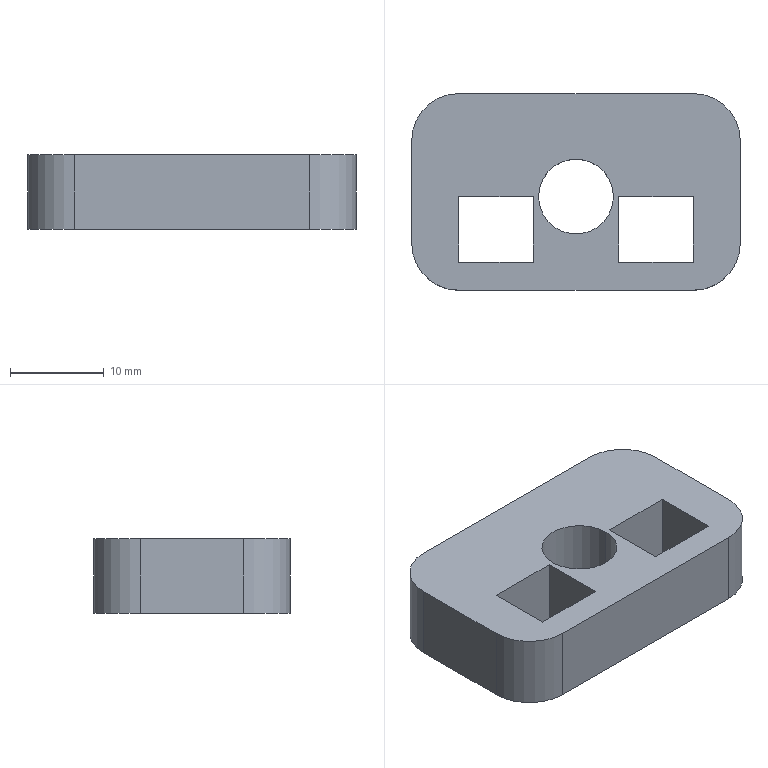Part | SolidWorks | features Fillet 1, FlatPattern 1, SMBaseFlange 1, SheetMetal 1 | 1 solid | 20 faces | box 35.1 x 21 x 8 mm | volume 4427 mm3 | plane 14 | cylinder 6 | commonest cylinder face diameters 10 x4 8 x2
STEP:
#1=CARTESIAN_POINT('',(8.55,26.043,8.));
#2=VERTEX_POINT('',#1);
#3=CARTESIAN_POINT('',(16.55,26.043,8.));
#4=VERTEX_POINT('',#3);
#5=CARTESIAN_POINT('',(12.55,26.043,8.));
#6=DIRECTION('',(0.,0.,1.));
#7=DIRECTION('',(1.,0.,0.));
#8=AXIS2_PLACEMENT_3D('',#5,#6,#7);
#9=CIRCLE('',#8,4.);
#10=EDGE_CURVE('',#2,#4,#9,.T.);
#11=ORIENTED_EDGE('',*,*,#10,.T.);
#12=CARTESIAN_POINT('',(16.55,26.043,0.));
#13=VERTEX_POINT('',#12);
#14=CARTESIAN_POINT('',(16.55,26.043,8.));
#15=DIRECTION('',(0.,0.,-1.));
#16=VECTOR('',#15,1000.);
#17=LINE('',#14,#16);
#18=EDGE_CURVE('',#4,#13,#17,.T.);
#19=ORIENTED_EDGE('',*,*,#18,.T.);
#20=CARTESIAN_POINT('',(8.55,26.043,0.));
#21=VERTEX_POINT('',#20);
#22=CARTESIAN_POINT('',(12.55,26.043,0.));
#23=DIRECTION('',(0.,0.,1.));
#24=DIRECTION('',(1.,0.,0.));
#25=AXIS2_PLACEMENT_3D('',#22,#23,#24);
#26=CIRCLE('',#25,4.);
#27=EDGE_CURVE('',#21,#13,#26,.T.);
#28=ORIENTED_EDGE('',*,*,#27,.F.);
#29=CARTESIAN_POINT('',(8.55,26.043,8.));
#30=DIRECTION('',(0.,0.,-1.));
#31=VECTOR('',#30,1000.);
#32=LINE('',#29,#31);
#33=EDGE_CURVE('',#2,#21,#32,.T.);
#34=ORIENTED_EDGE('',*,*,#33,.F.);
#35=EDGE_LOOP('',(#11,#19,#28,#34));
#36=FACE_OUTER_BOUND('',#35,.T.);
#37=CARTESIAN_POINT('',(12.55,26.043,8.));
#38=DIRECTION('',(0.,0.,-1.));
#39=DIRECTION('',(-1.,0.,0.));
#40=AXIS2_PLACEMENT_3D('',#37,#38,#39);
#41=CYLINDRICAL_SURFACE('',#40,4.);
#42=ADVANCED_FACE('',(#36),#41,.F.);
#43=CARTESIAN_POINT('',(0.,26.043,8.));
#44=VERTEX_POINT('',#43);
#45=CARTESIAN_POINT('',(0.,19.043,8.));
#46=VERTEX_POINT('',#45);
#47=CARTESIAN_POINT('',(0.,19.043,8.));
#48=DIRECTION('',(0.,-1.,0.));
#49=VECTOR('',#48,1000.);
#50=LINE('',#47,#49);
#51=EDGE_CURVE('',#44,#46,#50,.T.);
#52=ORIENTED_EDGE('',*,*,#51,.F.);
#53=CARTESIAN_POINT('',(8.,26.043,8.));
#54=VERTEX_POINT('',#53);
#55=CARTESIAN_POINT('',(0.,26.043,8.));
#56=DIRECTION('',(-1.,0.,0.));
#57=VECTOR('',#56,1000.);
#58=LINE('',#55,#57);
#59=EDGE_CURVE('',#54,#44,#58,.T.);
#60=ORIENTED_EDGE('',*,*,#59,.F.);
#61=CARTESIAN_POINT('',(8.,19.043,8.));
#62=VERTEX_POINT('',#61);
#63=CARTESIAN_POINT('',(8.,19.043,8.));
#64=DIRECTION('',(0.,1.,0.));
#65=VECTOR('',#64,1000.);
#66=LINE('',#63,#65);
#67=EDGE_CURVE('',#62,#54,#66,.T.);
#68=ORIENTED_EDGE('',*,*,#67,.F.);
#69=CARTESIAN_POINT('',(0.,19.043,8.));
#70=DIRECTION('',(1.,0.,0.));
#71=VECTOR('',#70,1000.);
#72=LINE('',#69,#71);
#73=EDGE_CURVE('',#46,#62,#72,.T.);
#74=ORIENTED_EDGE('',*,*,#73,.F.);
#75=EDGE_LOOP('',(#52,#60,#68,#74));
#76=FACE_BOUND('',#75,.T.);
#77=CARTESIAN_POINT('',(25.1,37.043,8.));
#78=VERTEX_POINT('',#77);
#79=CARTESIAN_POINT('',(0.,37.043,8.));
#80=VERTEX_POINT('',#79);
#81=CARTESIAN_POINT('',(-5.,37.043,8.));
#82=DIRECTION('',(-1.,0.,0.));
#83=VECTOR('',#82,1000.);
#84=LINE('',#81,#83);
#85=EDGE_CURVE('',#78,#80,#84,.T.);
#86=ORIENTED_EDGE('',*,*,#85,.T.);
#87=CARTESIAN_POINT('',(-5.,32.043,8.));
#88=VERTEX_POINT('',#87);
#89=CARTESIAN_POINT('',(0.,32.043,8.));
#90=DIRECTION('',(0.,0.,1.));
#91=DIRECTION('',(-1.,0.,0.));
#92=AXIS2_PLACEMENT_3D('',#89,#90,#91);
#93=CIRCLE('',#92,5.);
#94=EDGE_CURVE('',#80,#88,#93,.T.);
#95=ORIENTED_EDGE('',*,*,#94,.T.);
#96=CARTESIAN_POINT('',(-5.,21.043,8.));
#97=VERTEX_POINT('',#96);
#98=CARTESIAN_POINT('',(-5.,16.043,8.));
#99=DIRECTION('',(0.,-1.,0.));
#100=VECTOR('',#99,1000.);
#101=LINE('',#98,#100);
#102=EDGE_CURVE('',#88,#97,#101,.T.);
#103=ORIENTED_EDGE('',*,*,#102,.T.);
#104=CARTESIAN_POINT('',(0.,16.043,8.));
#105=VERTEX_POINT('',#104);
#106=CARTESIAN_POINT('',(0.,21.043,8.));
#107=DIRECTION('',(0.,0.,1.));
#108=DIRECTION('',(-1.,0.,0.));
#109=AXIS2_PLACEMENT_3D('',#106,#107,#108);
#110=CIRCLE('',#109,5.);
#111=EDGE_CURVE('',#97,#105,#110,.T.);
#112=ORIENTED_EDGE('',*,*,#111,.T.);
#113=CARTESIAN_POINT('',(25.1,16.043,8.));
#114=VERTEX_POINT('',#113);
#115=CARTESIAN_POINT('',(-5.,16.043,8.));
#116=DIRECTION('',(1.,0.,0.));
#117=VECTOR('',#116,1000.);
#118=LINE('',#115,#117);
#119=EDGE_CURVE('',#105,#114,#118,.T.);
#120=ORIENTED_EDGE('',*,*,#119,.T.);
#121=CARTESIAN_POINT('',(30.1,21.043,8.));
#122=VERTEX_POINT('',#121);
#123=CARTESIAN_POINT('',(25.1,21.043,8.));
#124=DIRECTION('',(0.,0.,1.));
#125=DIRECTION('',(-1.,0.,0.));
#126=AXIS2_PLACEMENT_3D('',#123,#124,#125);
#127=CIRCLE('',#126,5.);
#128=EDGE_CURVE('',#114,#122,#127,.T.);
#129=ORIENTED_EDGE('',*,*,#128,.T.);
#130=CARTESIAN_POINT('',(30.1,32.043,8.));
#131=VERTEX_POINT('',#130);
#132=CARTESIAN_POINT('',(30.1,16.043,8.));
#133=DIRECTION('',(0.,1.,0.));
#134=VECTOR('',#133,1000.);
#135=LINE('',#132,#134);
#136=EDGE_CURVE('',#122,#131,#135,.T.);
#137=ORIENTED_EDGE('',*,*,#136,.T.);
#138=CARTESIAN_POINT('',(25.1,32.043,8.));
#139=DIRECTION('',(0.,0.,1.));
#140=DIRECTION('',(-1.,0.,0.));
#141=AXIS2_PLACEMENT_3D('',#138,#139,#140);
#142=CIRCLE('',#141,5.);
#143=EDGE_CURVE('',#131,#78,#142,.T.);
#144=ORIENTED_EDGE('',*,*,#143,.T.);
#145=EDGE_LOOP('',(#86,#95,#103,#112,#120,#129,#137,#144));
#146=FACE_OUTER_BOUND('',#145,.T.);
#147=CARTESIAN_POINT('',(17.1,26.043,8.));
#148=VERTEX_POINT('',#147);
#149=CARTESIAN_POINT('',(17.1,19.043,8.));
#150=VERTEX_POINT('',#149);
#151=CARTESIAN_POINT('',(17.1,19.043,8.));
#152=DIRECTION('',(0.,-1.,0.));
#153=VECTOR('',#152,1000.);
#154=LINE('',#151,#153);
#155=EDGE_CURVE('',#148,#150,#154,.T.);
#156=ORIENTED_EDGE('',*,*,#155,.F.);
#157=CARTESIAN_POINT('',(25.1,26.043,8.));
#158=VERTEX_POINT('',#157);
#159=CARTESIAN_POINT('',(17.1,26.043,8.));
#160=DIRECTION('',(-1.,0.,0.));
#161=VECTOR('',#160,1000.);
#162=LINE('',#159,#161);
#163=EDGE_CURVE('',#158,#148,#162,.T.);
#164=ORIENTED_EDGE('',*,*,#163,.F.);
#165=CARTESIAN_POINT('',(25.1,19.043,8.));
#166=VERTEX_POINT('',#165);
#167=CARTESIAN_POINT('',(25.1,19.043,8.));
#168=DIRECTION('',(0.,1.,0.));
#169=VECTOR('',#168,1000.);
#170=LINE('',#167,#169);
#171=EDGE_CURVE('',#166,#158,#170,.T.);
#172=ORIENTED_EDGE('',*,*,#171,.F.);
#173=CARTESIAN_POINT('',(17.1,19.043,8.));
#174=DIRECTION('',(1.,0.,0.));
#175=VECTOR('',#174,1000.);
#176=LINE('',#173,#175);
#177=EDGE_CURVE('',#150,#166,#176,.T.);
#178=ORIENTED_EDGE('',*,*,#177,.F.);
#179=EDGE_LOOP('',(#156,#164,#172,#178));
#180=FACE_BOUND('',#179,.T.);
#181=ORIENTED_EDGE('',*,*,#10,.F.);
#182=CARTESIAN_POINT('',(12.55,26.043,8.));
#183=DIRECTION('',(0.,0.,1.));
#184=DIRECTION('',(1.,0.,0.));
#185=AXIS2_PLACEMENT_3D('',#182,#183,#184);
#186=CIRCLE('',#185,4.);
#187=EDGE_CURVE('',#4,#2,#186,.T.);
#188=ORIENTED_EDGE('',*,*,#187,.F.);
#189=EDGE_LOOP('',(#181,#188));
#190=FACE_BOUND('',#189,.T.);
#191=CARTESIAN_POINT('',(0.,0.,8.));
#192=DIRECTION('',(0.,0.,-1.));
#193=DIRECTION('',(-1.,0.,0.));
#194=AXIS2_PLACEMENT_3D('',#191,#192,#193);
#195=PLANE('',#194);
#196=ADVANCED_FACE('',(#76,#146,#180,#190),#195,.F.);
#197=CARTESIAN_POINT('',(25.1,26.043,0.));
#198=VERTEX_POINT('',#197);
#199=CARTESIAN_POINT('',(17.1,26.043,0.));
#200=VERTEX_POINT('',#199);
#201=CARTESIAN_POINT('',(17.1,26.043,0.));
#202=DIRECTION('',(-1.,0.,0.));
#203=VECTOR('',#202,1000.);
#204=LINE('',#201,#203);
#205=EDGE_CURVE('',#198,#200,#204,.T.);
#206=ORIENTED_EDGE('',*,*,#205,.T.);
#207=CARTESIAN_POINT('',(17.1,19.043,0.));
#208=VERTEX_POINT('',#207);
#209=CARTESIAN_POINT('',(17.1,19.043,0.));
#210=DIRECTION('',(0.,-1.,0.));
#211=VECTOR('',#210,1000.);
#212=LINE('',#209,#211);
#213=EDGE_CURVE('',#200,#208,#212,.T.);
#214=ORIENTED_EDGE('',*,*,#213,.T.);
#215=CARTESIAN_POINT('',(25.1,19.043,0.));
#216=VERTEX_POINT('',#215);
#217=CARTESIAN_POINT('',(17.1,19.043,0.));
#218=DIRECTION('',(1.,0.,0.));
#219=VECTOR('',#218,1000.);
#220=LINE('',#217,#219);
#221=EDGE_CURVE('',#208,#216,#220,.T.);
#222=ORIENTED_EDGE('',*,*,#221,.T.);
#223=CARTESIAN_POINT('',(25.1,19.043,0.));
#224=DIRECTION('',(0.,1.,0.));
#225=VECTOR('',#224,1000.);
#226=LINE('',#223,#225);
#227=EDGE_CURVE('',#216,#198,#226,.T.);
#228=ORIENTED_EDGE('',*,*,#227,.T.);
#229=EDGE_LOOP('',(#206,#214,#222,#228));
#230=FACE_BOUND('',#229,.T.);
#231=CARTESIAN_POINT('',(8.,26.043,0.));
#232=VERTEX_POINT('',#231);
#233=CARTESIAN_POINT('',(0.,26.043,0.));
#234=VERTEX_POINT('',#233);
#235=CARTESIAN_POINT('',(0.,26.043,0.));
#236=DIRECTION('',(-1.,0.,0.));
#237=VECTOR('',#236,1000.);
#238=LINE('',#235,#237);
#239=EDGE_CURVE('',#232,#234,#238,.T.);
#240=ORIENTED_EDGE('',*,*,#239,.T.);
#241=CARTESIAN_POINT('',(0.,19.043,0.));
#242=VERTEX_POINT('',#241);
#243=CARTESIAN_POINT('',(0.,19.043,0.));
#244=DIRECTION('',(0.,-1.,0.));
#245=VECTOR('',#244,1000.);
#246=LINE('',#243,#245);
#247=EDGE_CURVE('',#234,#242,#246,.T.);
#248=ORIENTED_EDGE('',*,*,#247,.T.);
#249=CARTESIAN_POINT('',(8.,19.043,0.));
#250=VERTEX_POINT('',#249);
#251=CARTESIAN_POINT('',(0.,19.043,0.));
#252=DIRECTION('',(1.,0.,0.));
#253=VECTOR('',#252,1000.);
#254=LINE('',#251,#253);
#255=EDGE_CURVE('',#242,#250,#254,.T.);
#256=ORIENTED_EDGE('',*,*,#255,.T.);
#257=CARTESIAN_POINT('',(8.,19.043,0.));
#258=DIRECTION('',(0.,1.,0.));
#259=VECTOR('',#258,1000.);
#260=LINE('',#257,#259);
#261=EDGE_CURVE('',#250,#232,#260,.T.);
#262=ORIENTED_EDGE('',*,*,#261,.T.);
#263=EDGE_LOOP('',(#240,#248,#256,#262));
#264=FACE_BOUND('',#263,.T.);
#265=CARTESIAN_POINT('',(-5.,32.043,0.));
#266=VERTEX_POINT('',#265);
#267=CARTESIAN_POINT('',(-5.,21.043,0.));
#268=VERTEX_POINT('',#267);
#269=CARTESIAN_POINT('',(-5.,16.043,0.));
#270=DIRECTION('',(0.,-1.,0.));
#271=VECTOR('',#270,1000.);
#272=LINE('',#269,#271);
#273=EDGE_CURVE('',#266,#268,#272,.T.);
#274=ORIENTED_EDGE('',*,*,#273,.F.);
#275=CARTESIAN_POINT('',(0.,37.043,0.));
#276=VERTEX_POINT('',#275);
#277=CARTESIAN_POINT('',(0.,32.043,0.));
#278=DIRECTION('',(0.,0.,-1.));
#279=DIRECTION('',(-1.,0.,0.));
#280=AXIS2_PLACEMENT_3D('',#277,#278,#279);
#281=CIRCLE('',#280,5.);
#282=EDGE_CURVE('',#266,#276,#281,.T.);
#283=ORIENTED_EDGE('',*,*,#282,.T.);
#284=CARTESIAN_POINT('',(25.1,37.043,0.));
#285=VERTEX_POINT('',#284);
#286=CARTESIAN_POINT('',(-5.,37.043,0.));
#287=DIRECTION('',(-1.,0.,0.));
#288=VECTOR('',#287,1000.);
#289=LINE('',#286,#288);
#290=EDGE_CURVE('',#285,#276,#289,.T.);
#291=ORIENTED_EDGE('',*,*,#290,.F.);
#292=CARTESIAN_POINT('',(30.1,32.043,0.));
#293=VERTEX_POINT('',#292);
#294=CARTESIAN_POINT('',(25.1,32.043,0.));
#295=DIRECTION('',(0.,0.,-1.));
#296=DIRECTION('',(-1.,0.,0.));
#297=AXIS2_PLACEMENT_3D('',#294,#295,#296);
#298=CIRCLE('',#297,5.);
#299=EDGE_CURVE('',#285,#293,#298,.T.);
#300=ORIENTED_EDGE('',*,*,#299,.T.);
#301=CARTESIAN_POINT('',(30.1,21.043,0.));
#302=VERTEX_POINT('',#301);
#303=CARTESIAN_POINT('',(30.1,16.043,0.));
#304=DIRECTION('',(0.,1.,0.));
#305=VECTOR('',#304,1000.);
#306=LINE('',#303,#305);
#307=EDGE_CURVE('',#302,#293,#306,.T.);
#308=ORIENTED_EDGE('',*,*,#307,.F.);
#309=CARTESIAN_POINT('',(25.1,16.043,0.));
#310=VERTEX_POINT('',#309);
#311=CARTESIAN_POINT('',(25.1,21.043,0.));
#312=DIRECTION('',(0.,0.,-1.));
#313=DIRECTION('',(-1.,0.,0.));
#314=AXIS2_PLACEMENT_3D('',#311,#312,#313);
#315=CIRCLE('',#314,5.);
#316=EDGE_CURVE('',#302,#310,#315,.T.);
#317=ORIENTED_EDGE('',*,*,#316,.T.);
#318=CARTESIAN_POINT('',(0.,16.043,0.));
#319=VERTEX_POINT('',#318);
#320=CARTESIAN_POINT('',(-5.,16.043,0.));
#321=DIRECTION('',(1.,0.,0.));
#322=VECTOR('',#321,1000.);
#323=LINE('',#320,#322);
#324=EDGE_CURVE('',#319,#310,#323,.T.);
#325=ORIENTED_EDGE('',*,*,#324,.F.);
#326=CARTESIAN_POINT('',(0.,21.043,0.));
#327=DIRECTION('',(0.,0.,-1.));
#328=DIRECTION('',(-1.,0.,0.));
#329=AXIS2_PLACEMENT_3D('',#326,#327,#328);
#330=CIRCLE('',#329,5.);
#331=EDGE_CURVE('',#319,#268,#330,.T.);
#332=ORIENTED_EDGE('',*,*,#331,.T.);
#333=EDGE_LOOP('',(#274,#283,#291,#300,#308,#317,#325,#332));
#334=FACE_OUTER_BOUND('',#333,.T.);
#335=ORIENTED_EDGE('',*,*,#27,.T.);
#336=CARTESIAN_POINT('',(12.55,26.043,0.));
#337=DIRECTION('',(0.,0.,1.));
#338=DIRECTION('',(1.,0.,0.));
#339=AXIS2_PLACEMENT_3D('',#336,#337,#338);
#340=CIRCLE('',#339,4.);
#341=EDGE_CURVE('',#13,#21,#340,.T.);
#342=ORIENTED_EDGE('',*,*,#341,.T.);
#343=EDGE_LOOP('',(#335,#342));
#344=FACE_BOUND('',#343,.T.);
#345=CARTESIAN_POINT('',(0.,0.,0.));
#346=DIRECTION('',(0.,0.,-1.));
#347=DIRECTION('',(-1.,0.,0.));
#348=AXIS2_PLACEMENT_3D('',#345,#346,#347);
#349=PLANE('',#348);
#350=ADVANCED_FACE('',(#230,#264,#334,#344),#349,.T.);
#351=ORIENTED_EDGE('',*,*,#102,.F.);
#352=CARTESIAN_POINT('',(-5.,32.043,8.));
#353=DIRECTION('',(0.,0.,-1.));
#354=VECTOR('',#353,1000.);
#355=LINE('',#352,#354);
#356=EDGE_CURVE('',#88,#266,#355,.T.);
#357=ORIENTED_EDGE('',*,*,#356,.T.);
#358=ORIENTED_EDGE('',*,*,#273,.T.);
#359=CARTESIAN_POINT('',(-5.,21.043,8.));
#360=DIRECTION('',(0.,0.,1.));
#361=VECTOR('',#360,1000.);
#362=LINE('',#359,#361);
#363=EDGE_CURVE('',#268,#97,#362,.T.);
#364=ORIENTED_EDGE('',*,*,#363,.T.);
#365=EDGE_LOOP('',(#351,#357,#358,#364));
#366=FACE_OUTER_BOUND('',#365,.T.);
#367=CARTESIAN_POINT('',(-5.,16.043,8.));
#368=DIRECTION('',(1.,0.,0.));
#369=DIRECTION('',(0.,1.,0.));
#370=AXIS2_PLACEMENT_3D('',#367,#368,#369);
#371=PLANE('',#370);
#372=ADVANCED_FACE('',(#366),#371,.F.);
#373=ORIENTED_EDGE('',*,*,#324,.T.);
#374=CARTESIAN_POINT('',(25.1,16.043,8.));
#375=DIRECTION('',(0.,0.,1.));
#376=VECTOR('',#375,1000.);
#377=LINE('',#374,#376);
#378=EDGE_CURVE('',#310,#114,#377,.T.);
#379=ORIENTED_EDGE('',*,*,#378,.T.);
#380=ORIENTED_EDGE('',*,*,#119,.F.);
#381=CARTESIAN_POINT('',(0.,16.043,8.));
#382=DIRECTION('',(0.,0.,-1.));
#383=VECTOR('',#382,1000.);
#384=LINE('',#381,#383);
#385=EDGE_CURVE('',#105,#319,#384,.T.);
#386=ORIENTED_EDGE('',*,*,#385,.T.);
#387=EDGE_LOOP('',(#373,#379,#380,#386));
#388=FACE_OUTER_BOUND('',#387,.T.);
#389=CARTESIAN_POINT('',(-5.,16.043,8.));
#390=DIRECTION('',(0.,1.,0.));
#391=DIRECTION('',(0.,0.,1.));
#392=AXIS2_PLACEMENT_3D('',#389,#390,#391);
#393=PLANE('',#392);
#394=ADVANCED_FACE('',(#388),#393,.F.);
#395=ORIENTED_EDGE('',*,*,#307,.T.);
#396=CARTESIAN_POINT('',(30.1,32.043,8.));
#397=DIRECTION('',(0.,0.,1.));
#398=VECTOR('',#397,1000.);
#399=LINE('',#396,#398);
#400=EDGE_CURVE('',#293,#131,#399,.T.);
#401=ORIENTED_EDGE('',*,*,#400,.T.);
#402=ORIENTED_EDGE('',*,*,#136,.F.);
#403=CARTESIAN_POINT('',(30.1,21.043,8.));
#404=DIRECTION('',(0.,0.,-1.));
#405=VECTOR('',#404,1000.);
#406=LINE('',#403,#405);
#407=EDGE_CURVE('',#122,#302,#406,.T.);
#408=ORIENTED_EDGE('',*,*,#407,.T.);
#409=EDGE_LOOP('',(#395,#401,#402,#408));
#410=FACE_OUTER_BOUND('',#409,.T.);
#411=CARTESIAN_POINT('',(30.1,16.043,8.));
#412=DIRECTION('',(-1.,0.,0.));
#413=DIRECTION('',(0.,0.,1.));
#414=AXIS2_PLACEMENT_3D('',#411,#412,#413);
#415=PLANE('',#414);
#416=ADVANCED_FACE('',(#410),#415,.F.);
#417=ORIENTED_EDGE('',*,*,#290,.T.);
#418=CARTESIAN_POINT('',(0.,37.043,8.));
#419=DIRECTION('',(0.,0.,1.));
#420=VECTOR('',#419,1000.);
#421=LINE('',#418,#420);
#422=EDGE_CURVE('',#276,#80,#421,.T.);
#423=ORIENTED_EDGE('',*,*,#422,.T.);
#424=ORIENTED_EDGE('',*,*,#85,.F.);
#425=CARTESIAN_POINT('',(25.1,37.043,8.));
#426=DIRECTION('',(0.,0.,-1.));
#427=VECTOR('',#426,1000.);
#428=LINE('',#425,#427);
#429=EDGE_CURVE('',#78,#285,#428,.T.);
#430=ORIENTED_EDGE('',*,*,#429,.T.);
#431=EDGE_LOOP('',(#417,#423,#424,#430));
#432=FACE_OUTER_BOUND('',#431,.T.);
#433=CARTESIAN_POINT('',(-5.,37.043,8.));
#434=DIRECTION('',(0.,-1.,0.));
#435=DIRECTION('',(0.,0.,-1.));
#436=AXIS2_PLACEMENT_3D('',#433,#434,#435);
#437=PLANE('',#436);
#438=ADVANCED_FACE('',(#432),#437,.F.);
#439=ORIENTED_EDGE('',*,*,#247,.F.);
#440=CARTESIAN_POINT('',(0.,26.043,8.));
#441=DIRECTION('',(0.,0.,-1.));
#442=VECTOR('',#441,1000.);
#443=LINE('',#440,#442);
#444=EDGE_CURVE('',#44,#234,#443,.T.);
#445=ORIENTED_EDGE('',*,*,#444,.F.);
#446=ORIENTED_EDGE('',*,*,#51,.T.);
#447=CARTESIAN_POINT('',(0.,19.043,8.));
#448=DIRECTION('',(0.,0.,-1.));
#449=VECTOR('',#448,1000.);
#450=LINE('',#447,#449);
#451=EDGE_CURVE('',#46,#242,#450,.T.);
#452=ORIENTED_EDGE('',*,*,#451,.T.);
#453=EDGE_LOOP('',(#439,#445,#446,#452));
#454=FACE_OUTER_BOUND('',#453,.T.);
#455=CARTESIAN_POINT('',(0.,19.043,8.));
#456=DIRECTION('',(1.,0.,0.));
#457=DIRECTION('',(0.,0.,-1.));
#458=AXIS2_PLACEMENT_3D('',#455,#456,#457);
#459=PLANE('',#458);
#460=ADVANCED_FACE('',(#454),#459,.T.);
#461=ORIENTED_EDGE('',*,*,#255,.F.);
#462=ORIENTED_EDGE('',*,*,#451,.F.);
#463=ORIENTED_EDGE('',*,*,#73,.T.);
#464=CARTESIAN_POINT('',(8.,19.043,8.));
#465=DIRECTION('',(0.,0.,-1.));
#466=VECTOR('',#465,1000.);
#467=LINE('',#464,#466);
#468=EDGE_CURVE('',#62,#250,#467,.T.);
#469=ORIENTED_EDGE('',*,*,#468,.T.);
#470=EDGE_LOOP('',(#461,#462,#463,#469));
#471=FACE_OUTER_BOUND('',#470,.T.);
#472=CARTESIAN_POINT('',(0.,19.043,8.));
#473=DIRECTION('',(0.,1.,0.));
#474=DIRECTION('',(0.,0.,1.));
#475=AXIS2_PLACEMENT_3D('',#472,#473,#474);
#476=PLANE('',#475);
#477=ADVANCED_FACE('',(#471),#476,.T.);
#478=ORIENTED_EDGE('',*,*,#261,.F.);
#479=ORIENTED_EDGE('',*,*,#468,.F.);
#480=ORIENTED_EDGE('',*,*,#67,.T.);
#481=CARTESIAN_POINT('',(8.,26.043,8.));
#482=DIRECTION('',(0.,0.,-1.));
#483=VECTOR('',#482,1000.);
#484=LINE('',#481,#483);
#485=EDGE_CURVE('',#54,#232,#484,.T.);
#486=ORIENTED_EDGE('',*,*,#485,.T.);
#487=EDGE_LOOP('',(#478,#479,#480,#486));
#488=FACE_OUTER_BOUND('',#487,.T.);
#489=CARTESIAN_POINT('',(8.,19.043,8.));
#490=DIRECTION('',(-1.,0.,0.));
#491=DIRECTION('',(0.,0.,1.));
#492=AXIS2_PLACEMENT_3D('',#489,#490,#491);
#493=PLANE('',#492);
#494=ADVANCED_FACE('',(#488),#493,.T.);
#495=ORIENTED_EDGE('',*,*,#239,.F.);
#496=ORIENTED_EDGE('',*,*,#485,.F.);
#497=ORIENTED_EDGE('',*,*,#59,.T.);
#498=ORIENTED_EDGE('',*,*,#444,.T.);
#499=EDGE_LOOP('',(#495,#496,#497,#498));
#500=FACE_OUTER_BOUND('',#499,.T.);
#501=CARTESIAN_POINT('',(0.,26.043,8.));
#502=DIRECTION('',(0.,-1.,0.));
#503=DIRECTION('',(0.,0.,-1.));
#504=AXIS2_PLACEMENT_3D('',#501,#502,#503);
#505=PLANE('',#504);
#506=ADVANCED_FACE('',(#500),#505,.T.);
#507=ORIENTED_EDGE('',*,*,#213,.F.);
#508=CARTESIAN_POINT('',(17.1,26.043,8.));
#509=DIRECTION('',(0.,0.,-1.));
#510=VECTOR('',#509,1000.);
#511=LINE('',#508,#510);
#512=EDGE_CURVE('',#148,#200,#511,.T.);
#513=ORIENTED_EDGE('',*,*,#512,.F.);
#514=ORIENTED_EDGE('',*,*,#155,.T.);
#515=CARTESIAN_POINT('',(17.1,19.043,8.));
#516=DIRECTION('',(0.,0.,-1.));
#517=VECTOR('',#516,1000.);
#518=LINE('',#515,#517);
#519=EDGE_CURVE('',#150,#208,#518,.T.);
#520=ORIENTED_EDGE('',*,*,#519,.T.);
#521=EDGE_LOOP('',(#507,#513,#514,#520));
#522=FACE_OUTER_BOUND('',#521,.T.);
#523=CARTESIAN_POINT('',(17.1,19.043,8.));
#524=DIRECTION('',(1.,0.,0.));
#525=DIRECTION('',(0.,0.,-1.));
#526=AXIS2_PLACEMENT_3D('',#523,#524,#525);
#527=PLANE('',#526);
#528=ADVANCED_FACE('',(#522),#527,.T.);
#529=ORIENTED_EDGE('',*,*,#221,.F.);
#530=ORIENTED_EDGE('',*,*,#519,.F.);
#531=ORIENTED_EDGE('',*,*,#177,.T.);
#532=CARTESIAN_POINT('',(25.1,19.043,8.));
#533=DIRECTION('',(0.,0.,-1.));
#534=VECTOR('',#533,1000.);
#535=LINE('',#532,#534);
#536=EDGE_CURVE('',#166,#216,#535,.T.);
#537=ORIENTED_EDGE('',*,*,#536,.T.);
#538=EDGE_LOOP('',(#529,#530,#531,#537));
#539=FACE_OUTER_BOUND('',#538,.T.);
#540=CARTESIAN_POINT('',(17.1,19.043,8.));
#541=DIRECTION('',(0.,1.,0.));
#542=DIRECTION('',(0.,0.,1.));
#543=AXIS2_PLACEMENT_3D('',#540,#541,#542);
#544=PLANE('',#543);
#545=ADVANCED_FACE('',(#539),#544,.T.);
#546=ORIENTED_EDGE('',*,*,#227,.F.);
#547=ORIENTED_EDGE('',*,*,#536,.F.);
#548=ORIENTED_EDGE('',*,*,#171,.T.);
#549=CARTESIAN_POINT('',(25.1,26.043,8.));
#550=DIRECTION('',(0.,0.,-1.));
#551=VECTOR('',#550,1000.);
#552=LINE('',#549,#551);
#553=EDGE_CURVE('',#158,#198,#552,.T.);
#554=ORIENTED_EDGE('',*,*,#553,.T.);
#555=EDGE_LOOP('',(#546,#547,#548,#554));
#556=FACE_OUTER_BOUND('',#555,.T.);
#557=CARTESIAN_POINT('',(25.1,19.043,8.));
#558=DIRECTION('',(-1.,0.,0.));
#559=DIRECTION('',(0.,0.,1.));
#560=AXIS2_PLACEMENT_3D('',#557,#558,#559);
#561=PLANE('',#560);
#562=ADVANCED_FACE('',(#556),#561,.T.);
#563=ORIENTED_EDGE('',*,*,#205,.F.);
#564=ORIENTED_EDGE('',*,*,#553,.F.);
#565=ORIENTED_EDGE('',*,*,#163,.T.);
#566=ORIENTED_EDGE('',*,*,#512,.T.);
#567=EDGE_LOOP('',(#563,#564,#565,#566));
#568=FACE_OUTER_BOUND('',#567,.T.);
#569=CARTESIAN_POINT('',(17.1,26.043,8.));
#570=DIRECTION('',(0.,-1.,0.));
#571=DIRECTION('',(0.,0.,-1.));
#572=AXIS2_PLACEMENT_3D('',#569,#570,#571);
#573=PLANE('',#572);
#574=ADVANCED_FACE('',(#568),#573,.T.);
#575=ORIENTED_EDGE('',*,*,#18,.F.);
#576=ORIENTED_EDGE('',*,*,#187,.T.);
#577=ORIENTED_EDGE('',*,*,#33,.T.);
#578=ORIENTED_EDGE('',*,*,#341,.F.);
#579=EDGE_LOOP('',(#575,#576,#577,#578));
#580=FACE_OUTER_BOUND('',#579,.T.);
#581=CARTESIAN_POINT('',(12.55,26.043,8.));
#582=DIRECTION('',(0.,0.,-1.));
#583=DIRECTION('',(-1.,0.,0.));
#584=AXIS2_PLACEMENT_3D('',#581,#582,#583);
#585=CYLINDRICAL_SURFACE('',#584,4.);
#586=ADVANCED_FACE('',(#580),#585,.F.);
#587=ORIENTED_EDGE('',*,*,#94,.F.);
#588=ORIENTED_EDGE('',*,*,#422,.F.);
#589=ORIENTED_EDGE('',*,*,#282,.F.);
#590=ORIENTED_EDGE('',*,*,#356,.F.);
#591=EDGE_LOOP('',(#587,#588,#589,#590));
#592=FACE_OUTER_BOUND('',#591,.T.);
#593=CARTESIAN_POINT('',(0.,32.043,8.));
#594=DIRECTION('',(0.,0.,-1.));
#595=DIRECTION('',(-1.,0.,0.));
#596=AXIS2_PLACEMENT_3D('',#593,#594,#595);
#597=CYLINDRICAL_SURFACE('',#596,5.);
#598=ADVANCED_FACE('',(#592),#597,.T.);
#599=ORIENTED_EDGE('',*,*,#143,.F.);
#600=ORIENTED_EDGE('',*,*,#400,.F.);
#601=ORIENTED_EDGE('',*,*,#299,.F.);
#602=ORIENTED_EDGE('',*,*,#429,.F.);
#603=EDGE_LOOP('',(#599,#600,#601,#602));
#604=FACE_OUTER_BOUND('',#603,.T.);
#605=CARTESIAN_POINT('',(25.1,32.043,8.));
#606=DIRECTION('',(0.,0.,-1.));
#607=DIRECTION('',(-1.,0.,0.));
#608=AXIS2_PLACEMENT_3D('',#605,#606,#607);
#609=CYLINDRICAL_SURFACE('',#608,5.);
#610=ADVANCED_FACE('',(#604),#609,.T.);
#611=ORIENTED_EDGE('',*,*,#128,.F.);
#612=ORIENTED_EDGE('',*,*,#378,.F.);
#613=ORIENTED_EDGE('',*,*,#316,.F.);
#614=ORIENTED_EDGE('',*,*,#407,.F.);
#615=EDGE_LOOP('',(#611,#612,#613,#614));
#616=FACE_OUTER_BOUND('',#615,.T.);
#617=CARTESIAN_POINT('',(25.1,21.043,8.));
#618=DIRECTION('',(0.,0.,-1.));
#619=DIRECTION('',(-1.,0.,0.));
#620=AXIS2_PLACEMENT_3D('',#617,#618,#619);
#621=CYLINDRICAL_SURFACE('',#620,5.);
#622=ADVANCED_FACE('',(#616),#621,.T.);
#623=ORIENTED_EDGE('',*,*,#111,.F.);
#624=ORIENTED_EDGE('',*,*,#363,.F.);
#625=ORIENTED_EDGE('',*,*,#331,.F.);
#626=ORIENTED_EDGE('',*,*,#385,.F.);
#627=EDGE_LOOP('',(#623,#624,#625,#626));
#628=FACE_OUTER_BOUND('',#627,.T.);
#629=CARTESIAN_POINT('',(0.,21.043,8.));
#630=DIRECTION('',(0.,0.,-1.));
#631=DIRECTION('',(-1.,0.,0.));
#632=AXIS2_PLACEMENT_3D('',#629,#630,#631);
#633=CYLINDRICAL_SURFACE('',#632,5.);
#634=ADVANCED_FACE('',(#628),#633,.T.);
#635=CLOSED_SHELL('',(#42,#196,#350,#372,#394,#416,#438,#460,#477,#494,#506,#528,#545,#562,#574,#586,#598,#610,#622,#634));
#636=MANIFOLD_SOLID_BREP('',#635);
#637=CARTESIAN_POINT('',(0.,0.,0.));
#638=DIRECTION('',(0.,0.,1.));
#639=DIRECTION('',(1.,0.,0.));
#640=AXIS2_PLACEMENT_3D('',#637,#638,#639);
#641=(LENGTH_UNIT()NAMED_UNIT(*)SI_UNIT(.MILLI.,.METRE.));
#642=UNCERTAINTY_MEASURE_WITH_UNIT(LENGTH_MEASURE(0.00001),#641,'','');
#643=(NAMED_UNIT(*)PLANE_ANGLE_UNIT()SI_UNIT($,.RADIAN.));
#644=(NAMED_UNIT(*)SI_UNIT($,.STERADIAN.)SOLID_ANGLE_UNIT());
#645=(GEOMETRIC_REPRESENTATION_CONTEXT(3)GLOBAL_UNCERTAINTY_ASSIGNED_CONTEXT((#642))GLOBAL_UNIT_ASSIGNED_CONTEXT((#641,#643,#644))REPRESENTATION_CONTEXT('',''));
#646=ADVANCED_BREP_SHAPE_REPRESENTATION('',(#636,#640),#645);